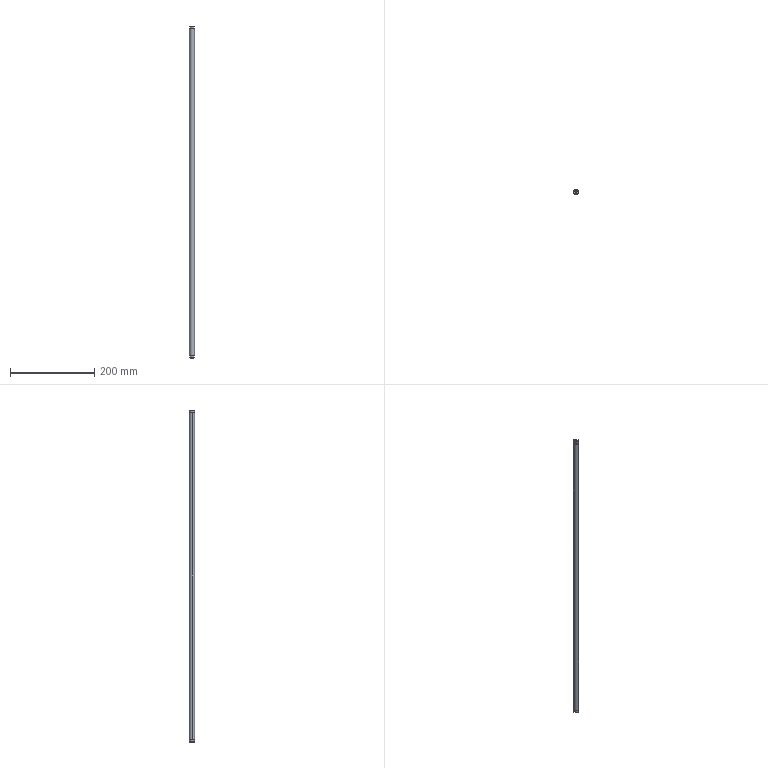Part | STEP file | Guide roller shaft 4 | 1 solid | 40 faces | box 12 x 12 x 790 mm | volume 88894 mm3 | cylinder 14 | plane 14 | cone 12 | commonest cylinder face diameters 12 x6 4.134 x4 11.5 x4